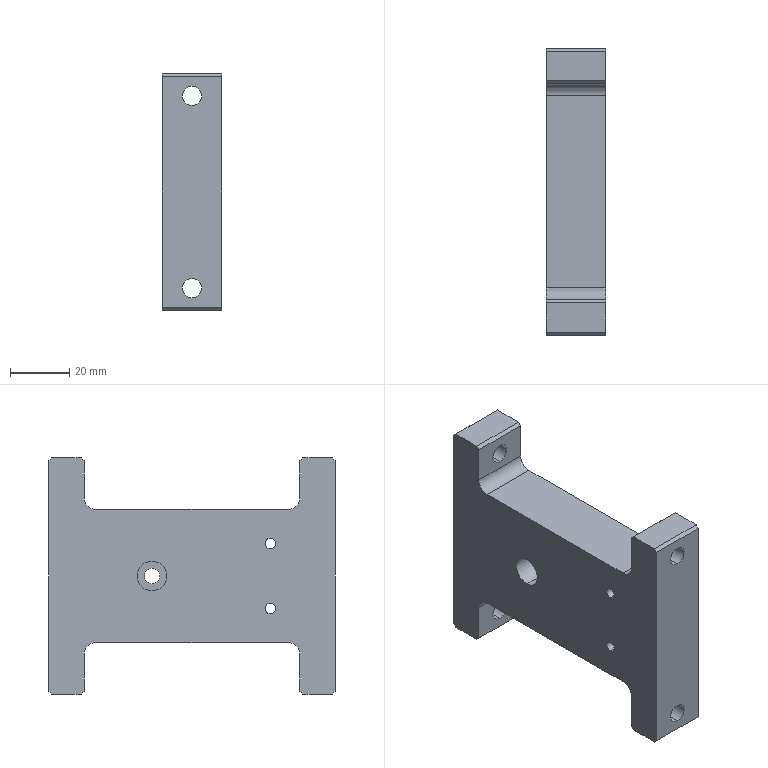Part | STEP file | Large support plate_sand-blasted, oxidised | 1 solid | 69 faces | box 20 x 97 x 80 mm | volume 92738 mm3 | cylinder 35 | plane 26 | cone 8 | commonest cylinder face diameters 3.3 x8 6.5 x8 3.5 x4 8 x4 22 x3 5.2 x2